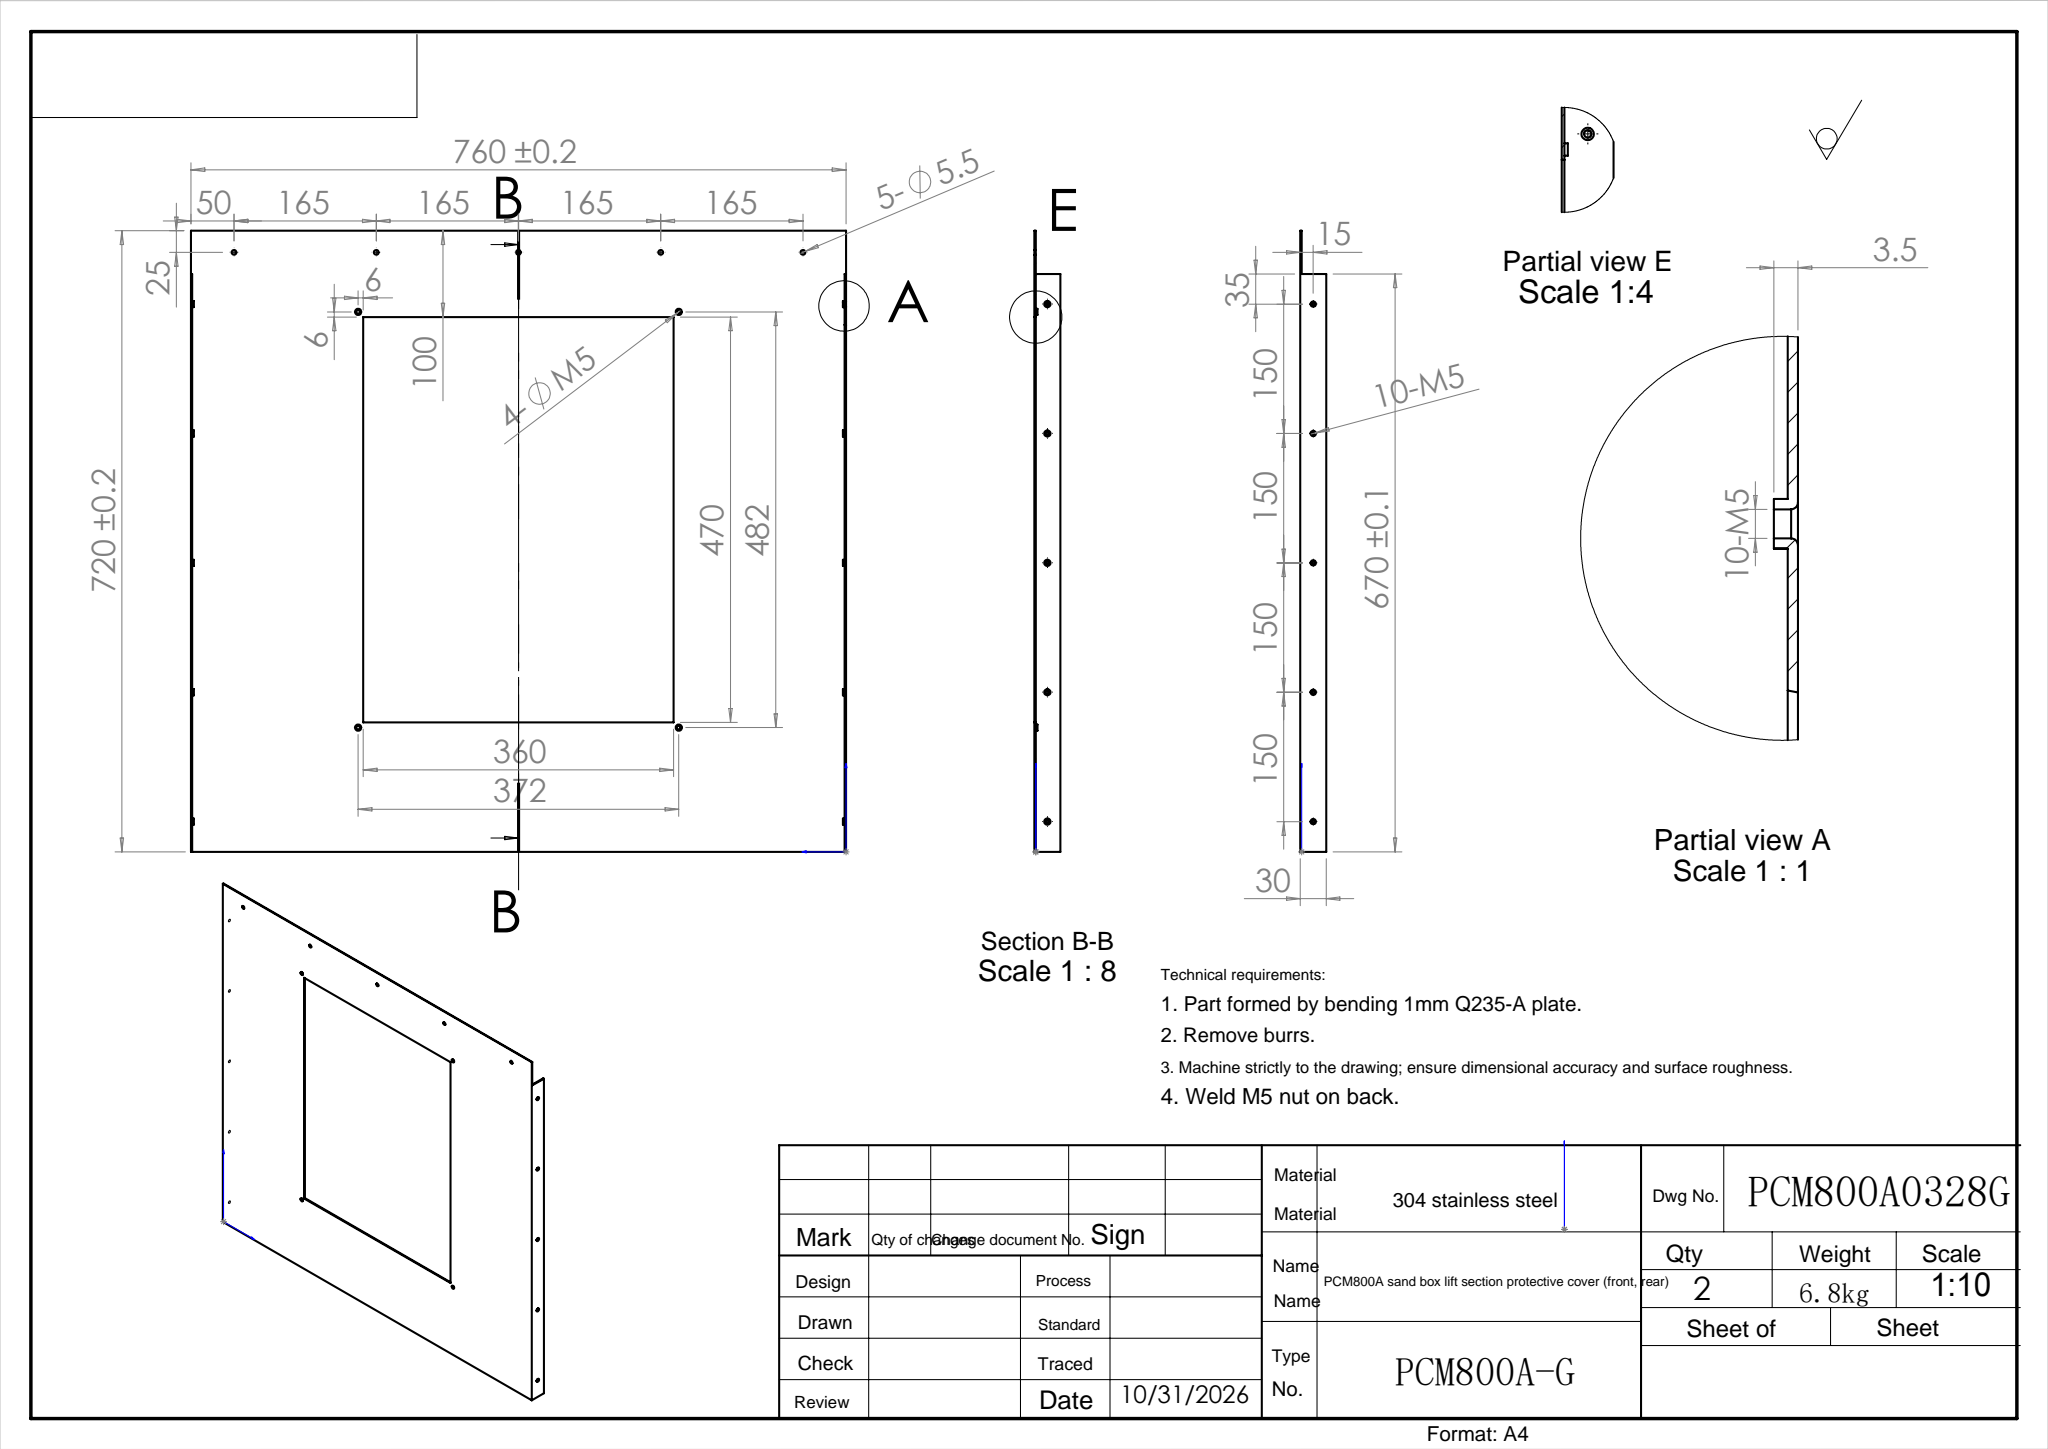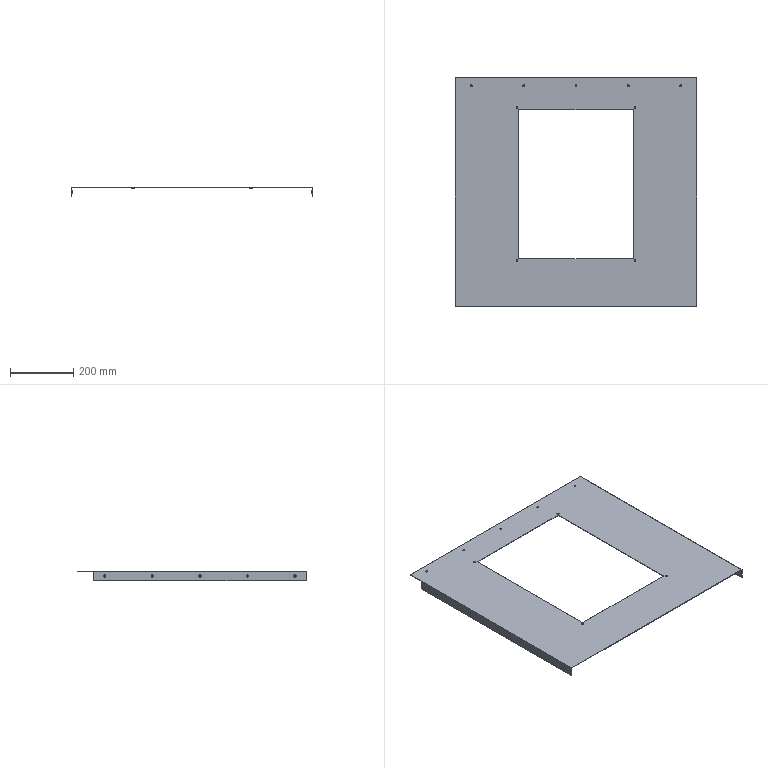Part | SolidWorks | features ICE 7, Fillet 2, Extrusion 1, HoleWzd 1 | 1 solid | 124 faces | box 760 x 720 x 30 mm | volume 624524 mm3 | cylinder 66 | plane 30 | torus 28 | commonest cylinder face diameters 4.2 x28 7.2 x28 5.5 x10